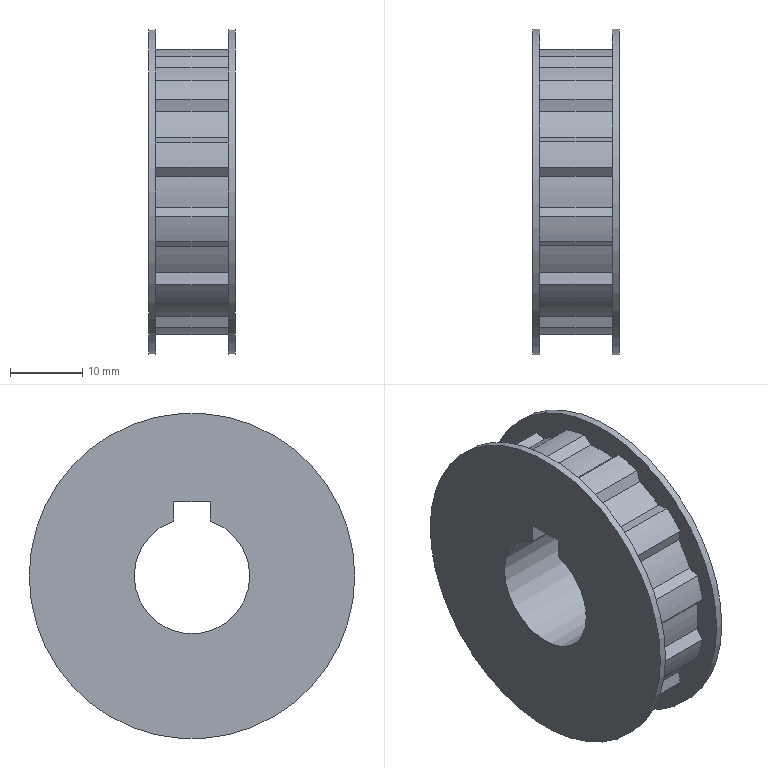Part | NX | features DATUM_CSYS 4, EXTRUDE 3, SKETCH 3, Container 1, EXTRACT_BODY 1, Geometry Instance 1, UNITE 1 | 1 solid | 58 faces | box 12 x 45 x 45 mm | volume 12364 mm3 | plane 31 | cylinder 27 | commonest cylinder face diameters 37.525 x12 40 x12 45 x2 16 x1